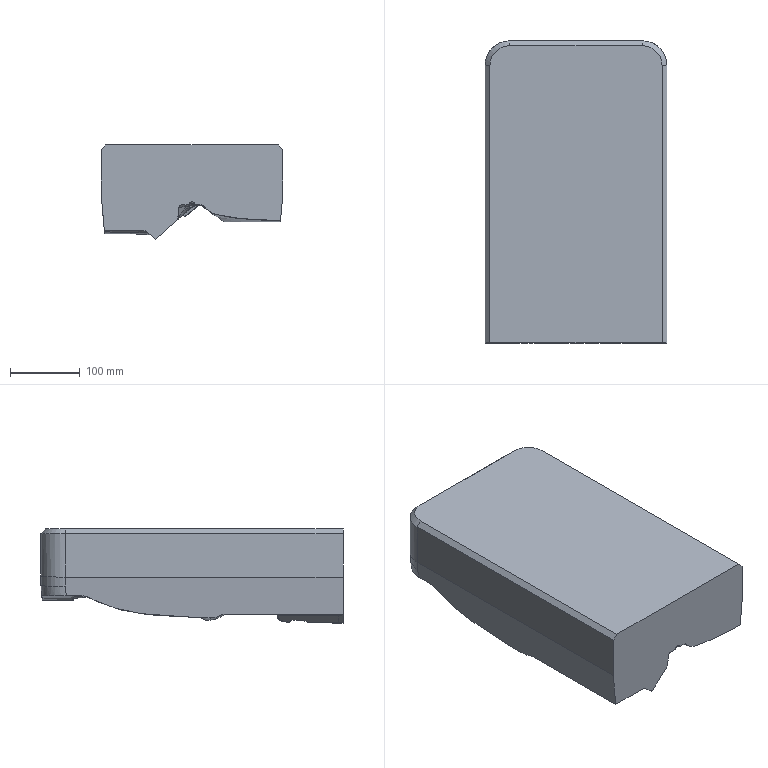Part | STEP file | 4-20.sldasm-Part-422 | 1 solid | 140 faces | box 260 x 432 x 134.618 mm | volume 11492972 mm3 | spline 99 | plane 24 | cylinder 15 | cone 2 | commonest cylinder face diameters 70 x6 12 x3 20 x3 4 x1 6 x1 24 x1